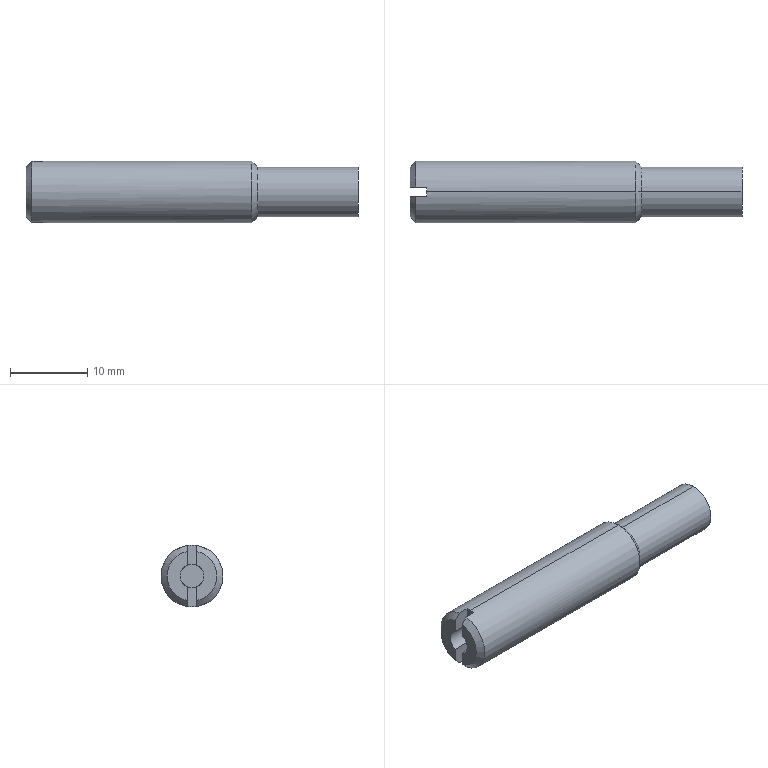Part | STEP file | 0217_Z_PJL8-10-1 | 1 solid | 30 faces | box 43 x 8 x 8 mm | volume 1284 mm3 | plane 18 | cylinder 8 | cone 4 | commonest cylinder face diameters 3.1 x2 4.8 x2 6.466 x2 8 x2